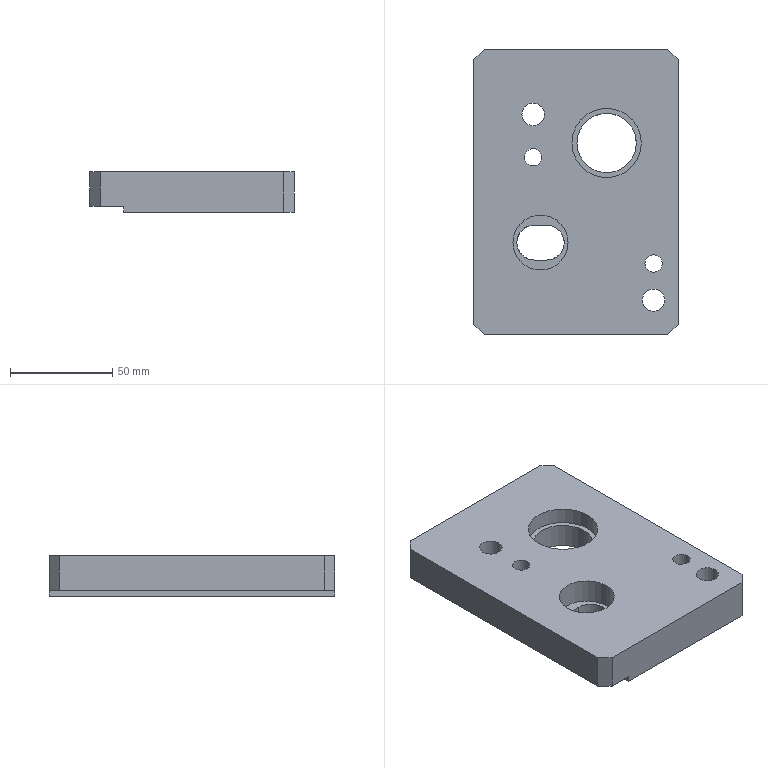Part | STEP file | lll_id3550_x_t | 1 solid | 33 faces | box 100 x 140 x 20 mm | volume 237831 mm3 | plane 20 | cylinder 11 | spline 2 | commonest cylinder face diameters 11 x4 8.5 x2 17 x2 27 x1 29.07 x1 34 x1
STEP:
#1=CARTESIAN_POINT('',(3254.117,145.288,22.5));
#2=VERTEX_POINT('',#1);
#3=CARTESIAN_POINT('',(3258.367,145.288,22.5));
#4=DIRECTION('',(0.,0.,-1.));
#5=DIRECTION('',(-1.,0.,0.));
#6=AXIS2_PLACEMENT_3D('',#3,#4,#5);
#7=CIRCLE('',#6,4.25);
#8=EDGE_CURVE('',#2,#2,#7,.T.);
#9=ORIENTED_EDGE('',*,*,#8,.T.);
#10=EDGE_LOOP('',(#9));
#11=FACE_BOUND('',#10,.T.);
#12=CARTESIAN_POINT('',(3195.117,197.288,22.5));
#13=VERTEX_POINT('',#12);
#14=CARTESIAN_POINT('',(3199.367,197.288,22.5));
#15=DIRECTION('',(0.,0.,-1.));
#16=DIRECTION('',(-1.,0.,0.));
#17=AXIS2_PLACEMENT_3D('',#14,#15,#16);
#18=CIRCLE('',#17,4.25);
#19=EDGE_CURVE('',#13,#13,#18,.T.);
#20=ORIENTED_EDGE('',*,*,#19,.T.);
#21=EDGE_LOOP('',(#20));
#22=FACE_BOUND('',#21,.T.);
#23=CARTESIAN_POINT('',(3252.867,127.288,22.5));
#24=VERTEX_POINT('',#23);
#25=CARTESIAN_POINT('',(3258.367,127.288,22.5));
#26=DIRECTION('',(0.,0.,-1.));
#27=DIRECTION('',(-1.,0.,0.));
#28=AXIS2_PLACEMENT_3D('',#25,#26,#27);
#29=CIRCLE('',#28,5.5);
#30=EDGE_CURVE('',#24,#24,#29,.T.);
#31=ORIENTED_EDGE('',*,*,#30,.T.);
#32=EDGE_LOOP('',(#31));
#33=FACE_BOUND('',#32,.T.);
#34=CARTESIAN_POINT('',(3270.367,115.288,22.5));
#35=VERTEX_POINT('',#34);
#36=CARTESIAN_POINT('',(3270.367,245.288,22.5));
#37=VERTEX_POINT('',#36);
#38=CARTESIAN_POINT('',(3270.367,195.288,22.5));
#39=DIRECTION('',(0.,1.,0.));
#40=VECTOR('',#39,1.);
#41=LINE('',#38,#40);
#42=EDGE_CURVE('',#35,#37,#41,.T.);
#43=ORIENTED_EDGE('',*,*,#42,.T.);
#44=CARTESIAN_POINT('',(3265.367,250.288,22.5));
#45=VERTEX_POINT('',#44);
#46=CARTESIAN_POINT('',(3443.404,72.251,22.5));
#47=DIRECTION('',(-0.7071,0.7071,0.));
#48=VECTOR('',#47,1.);
#49=LINE('',#46,#48);
#50=EDGE_CURVE('',#37,#45,#49,.T.);
#51=ORIENTED_EDGE('',*,*,#50,.T.);
#52=CARTESIAN_POINT('',(3175.367,250.288,22.5));
#53=VERTEX_POINT('',#52);
#54=CARTESIAN_POINT('',(3537.284,250.288,22.5));
#55=DIRECTION('',(-1.,0.,0.));
#56=VECTOR('',#55,1.);
#57=LINE('',#54,#56);
#58=EDGE_CURVE('',#45,#53,#57,.T.);
#59=ORIENTED_EDGE('',*,*,#58,.T.);
#60=CARTESIAN_POINT('',(3170.367,245.288,22.5));
#61=VERTEX_POINT('',#60);
#62=CARTESIAN_POINT('',(3314.247,389.168,22.5));
#63=DIRECTION('',(-0.7071,-0.7071,0.));
#64=VECTOR('',#63,1.);
#65=LINE('',#62,#64);
#66=EDGE_CURVE('',#53,#61,#65,.T.);
#67=ORIENTED_EDGE('',*,*,#66,.T.);
#68=CARTESIAN_POINT('',(3170.367,115.288,22.5));
#69=VERTEX_POINT('',#68);
#70=CARTESIAN_POINT('',(3170.367,166.13,22.5));
#71=DIRECTION('',(0.,1.,0.));
#72=VECTOR('',#71,1.);
#73=LINE('',#70,#72);
#74=EDGE_CURVE('',#69,#61,#73,.T.);
#75=ORIENTED_EDGE('',*,*,#74,.F.);
#76=CARTESIAN_POINT('',(3175.367,110.288,22.5));
#77=VERTEX_POINT('',#76);
#78=CARTESIAN_POINT('',(3328.404,-42.749,22.5));
#79=DIRECTION('',(0.7071,-0.7071,0.));
#80=VECTOR('',#79,1.);
#81=LINE('',#78,#80);
#82=EDGE_CURVE('',#69,#77,#81,.T.);
#83=ORIENTED_EDGE('',*,*,#82,.T.);
#84=CARTESIAN_POINT('',(3265.367,110.288,22.5));
#85=VERTEX_POINT('',#84);
#86=CARTESIAN_POINT('',(3537.284,110.288,22.5));
#87=DIRECTION('',(1.,0.,0.));
#88=VECTOR('',#87,1.);
#89=LINE('',#86,#88);
#90=EDGE_CURVE('',#77,#85,#89,.T.);
#91=ORIENTED_EDGE('',*,*,#90,.T.);
#92=CARTESIAN_POINT('',(3429.247,274.168,22.5));
#93=DIRECTION('',(0.7071,0.7071,0.));
#94=VECTOR('',#93,1.);
#95=LINE('',#92,#94);
#96=EDGE_CURVE('',#85,#35,#95,.T.);
#97=ORIENTED_EDGE('',*,*,#96,.T.);
#98=EDGE_LOOP('',(#43,#51,#59,#67,#75,#83,#91,#97));
#99=FACE_BOUND('',#98,.T.);
#100=CARTESIAN_POINT('',(3193.867,218.288,22.5));
#101=VERTEX_POINT('',#100);
#102=CARTESIAN_POINT('',(3199.367,218.288,22.5));
#103=DIRECTION('',(0.,0.,-1.));
#104=DIRECTION('',(-1.,0.,0.));
#105=AXIS2_PLACEMENT_3D('',#102,#103,#104);
#106=CIRCLE('',#105,5.5);
#107=EDGE_CURVE('',#101,#101,#106,.T.);
#108=ORIENTED_EDGE('',*,*,#107,.T.);
#109=EDGE_LOOP('',(#108));
#110=FACE_BOUND('',#109,.T.);
#111=CARTESIAN_POINT('',(3218.367,204.288,22.5));
#112=VERTEX_POINT('',#111);
#113=CARTESIAN_POINT('',(3235.367,204.288,22.5));
#114=DIRECTION('',(0.,0.,1.));
#115=DIRECTION('',(-1.,0.,0.));
#116=AXIS2_PLACEMENT_3D('',#113,#114,#115);
#117=CIRCLE('',#116,17.);
#118=EDGE_CURVE('',#112,#112,#117,.T.);
#119=ORIENTED_EDGE('',*,*,#118,.F.);
#120=EDGE_LOOP('',(#119));
#121=FACE_BOUND('',#120,.T.);
#122=CARTESIAN_POINT('',(3189.5,155.5,22.5));
#123=VERTEX_POINT('',#122);
#124=CARTESIAN_POINT('',(3203.,155.5,22.5));
#125=DIRECTION('',(0.,0.,-1.));
#126=DIRECTION('',(-1.,0.,0.));
#127=AXIS2_PLACEMENT_3D('',#124,#125,#126);
#128=CIRCLE('',#127,13.5);
#129=EDGE_CURVE('',#123,#123,#128,.T.);
#130=ORIENTED_EDGE('',*,*,#129,.T.);
#131=EDGE_LOOP('',(#130));
#132=FACE_BOUND('',#131,.T.);
#133=CARTESIAN_POINT('',(3537.284,166.13,22.5));
#134=DIRECTION('',(0.,0.,1.));
#135=DIRECTION('',(0.,-1.,0.));
#136=AXIS2_PLACEMENT_3D('',#133,#134,#135);
#137=PLANE('',#136);
#138=ADVANCED_FACE('',(#11,#22,#33,#99,#110,#121,#132),#137,.T.);
#139=CARTESIAN_POINT('',(3220.832,204.288,2.5));
#140=VERTEX_POINT('',#139);
#141=CARTESIAN_POINT('',(3235.367,204.288,2.5));
#142=DIRECTION('',(0.,0.,1.));
#143=DIRECTION('',(-1.,0.,0.));
#144=AXIS2_PLACEMENT_3D('',#141,#142,#143);
#145=CIRCLE('',#144,14.535);
#146=EDGE_CURVE('',#140,#140,#145,.T.);
#147=ORIENTED_EDGE('',*,*,#146,.F.);
#148=EDGE_LOOP('',(#147));
#149=FACE_BOUND('',#148,.T.);
#150=CARTESIAN_POINT('',(3220.832,204.288,14.5));
#151=VERTEX_POINT('',#150);
#152=CARTESIAN_POINT('',(3235.367,204.288,14.5));
#153=DIRECTION('',(0.,0.,1.));
#154=DIRECTION('',(-1.,0.,0.));
#155=AXIS2_PLACEMENT_3D('',#152,#153,#154);
#156=CIRCLE('',#155,14.535);
#157=EDGE_CURVE('',#151,#151,#156,.T.);
#158=ORIENTED_EDGE('',*,*,#157,.T.);
#159=EDGE_LOOP('',(#158));
#160=FACE_BOUND('',#159,.T.);
#161=CARTESIAN_POINT('',(3235.367,204.288,2.5));
#162=DIRECTION('',(0.000000008,0.,-1.));
#163=DIRECTION('',(1.,0.,0.000000008));
#164=AXIS2_PLACEMENT_3D('',#161,#162,#163);
#165=CYLINDRICAL_SURFACE('',#164,14.535);
#166=ADVANCED_FACE('',(#149,#160),#165,.F.);
#167=CARTESIAN_POINT('',(3206.065,146.965,10.5));
#168=VERTEX_POINT('',#167);
#169=CARTESIAN_POINT('',(3199.935,146.965,10.5));
#170=VERTEX_POINT('',#169);
#171=CARTESIAN_POINT('',(3214.,146.965,10.5));
#172=DIRECTION('',(-1.,0.,0.));
#173=VECTOR('',#172,1.);
#174=LINE('',#171,#173);
#175=EDGE_CURVE('',#168,#170,#174,.T.);
#176=ORIENTED_EDGE('',*,*,#175,.F.);
#177=CARTESIAN_POINT('',(3206.065,146.965,2.5));
#178=VERTEX_POINT('',#177);
#179=CARTESIAN_POINT('',(3206.065,146.965,2.5));
#180=DIRECTION('',(-0.000000008,0.,1.));
#181=VECTOR('',#180,1.);
#182=LINE('',#179,#181);
#183=EDGE_CURVE('',#178,#168,#182,.T.);
#184=ORIENTED_EDGE('',*,*,#183,.F.);
#185=CARTESIAN_POINT('',(3199.935,146.965,2.5));
#186=VERTEX_POINT('',#185);
#187=CARTESIAN_POINT('',(3214.,146.965,2.5));
#188=DIRECTION('',(1.,0.,0.));
#189=VECTOR('',#188,1.);
#190=LINE('',#187,#189);
#191=EDGE_CURVE('',#186,#178,#190,.T.);
#192=ORIENTED_EDGE('',*,*,#191,.F.);
#193=CARTESIAN_POINT('',(3199.935,146.965,2.5));
#194=DIRECTION('',(-0.000000008,0.,1.));
#195=VECTOR('',#194,1.);
#196=LINE('',#193,#195);
#197=EDGE_CURVE('',#186,#170,#196,.T.);
#198=ORIENTED_EDGE('',*,*,#197,.T.);
#199=EDGE_LOOP('',(#176,#184,#192,#198));
#200=FACE_OUTER_BOUND('',#199,.T.);
#201=CARTESIAN_POINT('',(3214.,146.965,2.5));
#202=DIRECTION('',(0.,1.,0.));
#203=DIRECTION('',(-1.,0.,-0.000000008));
#204=AXIS2_PLACEMENT_3D('',#201,#202,#203);
#205=PLANE('',#204);
#206=ADVANCED_FACE('',(#200),#205,.T.);
#207=CARTESIAN_POINT('',(3206.065,164.035,10.5));
#208=VERTEX_POINT('',#207);
#209=CARTESIAN_POINT('',(3206.065,164.035,10.5));
#210=CARTESIAN_POINT('',(3208.297,164.035,10.5));
#211=CARTESIAN_POINT('',(3210.515,163.121,10.5));
#212=CARTESIAN_POINT('',(3213.686,159.95,10.5));
#213=CARTESIAN_POINT('',(3214.6,157.741,10.5));
#214=CARTESIAN_POINT('',(3214.6,153.259,10.5));
#215=CARTESIAN_POINT('',(3213.685,151.05,10.5));
#216=CARTESIAN_POINT('',(3210.516,147.88,10.5));
#217=CARTESIAN_POINT('',(3208.297,146.965,10.5));
#218=CARTESIAN_POINT('',(3206.065,146.965,10.5));
#219=B_SPLINE_CURVE_WITH_KNOTS('',3,(#209,#210,#211,#212,#213,#214,#215,#216,#217,#218),.UNSPECIFIED.,.F.,.F.,(4,2,2,2,4),(0.,0.25,0.5,0.75,1.),.UNSPECIFIED.);
#220=EDGE_CURVE('',#208,#168,#219,.T.);
#221=ORIENTED_EDGE('',*,*,#220,.F.);
#222=CARTESIAN_POINT('',(3206.065,164.035,2.5));
#223=VERTEX_POINT('',#222);
#224=CARTESIAN_POINT('',(3206.065,164.035,2.5));
#225=DIRECTION('',(-0.000000008,0.,1.));
#226=VECTOR('',#225,1.);
#227=LINE('',#224,#226);
#228=EDGE_CURVE('',#223,#208,#227,.T.);
#229=ORIENTED_EDGE('',*,*,#228,.F.);
#230=CARTESIAN_POINT('',(3206.065,146.965,2.5));
#231=CARTESIAN_POINT('',(3208.297,146.965,2.5));
#232=CARTESIAN_POINT('',(3210.516,147.88,2.5));
#233=CARTESIAN_POINT('',(3213.685,151.05,2.5));
#234=CARTESIAN_POINT('',(3214.6,153.259,2.5));
#235=CARTESIAN_POINT('',(3214.6,157.741,2.5));
#236=CARTESIAN_POINT('',(3213.686,159.95,2.5));
#237=CARTESIAN_POINT('',(3210.515,163.121,2.5));
#238=CARTESIAN_POINT('',(3208.297,164.035,2.5));
#239=CARTESIAN_POINT('',(3206.065,164.035,2.5));
#240=B_SPLINE_CURVE_WITH_KNOTS('',3,(#230,#231,#232,#233,#234,#235,#236,#237,#238,#239),.UNSPECIFIED.,.F.,.F.,(4,2,2,2,4),(0.,0.25,0.5,0.75,1.),.UNSPECIFIED.);
#241=EDGE_CURVE('',#178,#223,#240,.T.);
#242=ORIENTED_EDGE('',*,*,#241,.F.);
#243=ORIENTED_EDGE('',*,*,#183,.T.);
#244=EDGE_LOOP('',(#221,#229,#242,#243));
#245=FACE_OUTER_BOUND('',#244,.T.);
#246=CARTESIAN_POINT('',(3206.065,164.035,1.5));
#247=CARTESIAN_POINT('',(3206.065,164.035,10.5));
#248=CARTESIAN_POINT('',(3208.297,164.035,1.5));
#249=CARTESIAN_POINT('',(3208.297,164.035,10.5));
#250=CARTESIAN_POINT('',(3210.515,163.121,1.5));
#251=CARTESIAN_POINT('',(3210.515,163.121,10.5));
#252=CARTESIAN_POINT('',(3213.686,159.95,1.5));
#253=CARTESIAN_POINT('',(3213.686,159.95,10.5));
#254=CARTESIAN_POINT('',(3214.6,157.741,1.5));
#255=CARTESIAN_POINT('',(3214.6,157.741,10.5));
#256=CARTESIAN_POINT('',(3214.6,153.259,1.5));
#257=CARTESIAN_POINT('',(3214.6,153.259,10.5));
#258=CARTESIAN_POINT('',(3213.685,151.05,1.5));
#259=CARTESIAN_POINT('',(3213.685,151.05,10.5));
#260=CARTESIAN_POINT('',(3210.516,147.88,1.5));
#261=CARTESIAN_POINT('',(3210.516,147.88,10.5));
#262=CARTESIAN_POINT('',(3208.297,146.965,1.5));
#263=CARTESIAN_POINT('',(3208.297,146.965,10.5));
#264=CARTESIAN_POINT('',(3206.065,146.965,1.5));
#265=CARTESIAN_POINT('',(3206.065,146.965,10.5));
#266=B_SPLINE_SURFACE_WITH_KNOTS('',3,1,((#246,#247),(#248,#249),(#250,#251),(#252,#253),(#254,#255),(#256,#257),(#258,#259),(#260,#261),(#262,#263),(#264,#265)),.UNSPECIFIED.,.F.,.F.,.F.,(4,2,2,2,4),(2,2),(0.,0.25,0.5,0.75,1.),(0.,1.),.UNSPECIFIED.);
#267=ADVANCED_FACE('',(#245),#266,.T.);
#268=CARTESIAN_POINT('',(3199.935,164.035,10.5));
#269=VERTEX_POINT('',#268);
#270=CARTESIAN_POINT('',(3214.,164.035,10.5));
#271=DIRECTION('',(1.,0.,0.));
#272=VECTOR('',#271,1.);
#273=LINE('',#270,#272);
#274=EDGE_CURVE('',#269,#208,#273,.T.);
#275=ORIENTED_EDGE('',*,*,#274,.F.);
#276=CARTESIAN_POINT('',(3199.935,164.035,2.5));
#277=VERTEX_POINT('',#276);
#278=CARTESIAN_POINT('',(3199.935,164.035,2.5));
#279=DIRECTION('',(-0.000000008,0.,1.));
#280=VECTOR('',#279,1.);
#281=LINE('',#278,#280);
#282=EDGE_CURVE('',#277,#269,#281,.T.);
#283=ORIENTED_EDGE('',*,*,#282,.F.);
#284=CARTESIAN_POINT('',(3214.,164.035,2.5));
#285=DIRECTION('',(-1.,0.,0.));
#286=VECTOR('',#285,1.);
#287=LINE('',#284,#286);
#288=EDGE_CURVE('',#223,#277,#287,.T.);
#289=ORIENTED_EDGE('',*,*,#288,.F.);
#290=ORIENTED_EDGE('',*,*,#228,.T.);
#291=EDGE_LOOP('',(#275,#283,#289,#290));
#292=FACE_OUTER_BOUND('',#291,.T.);
#293=CARTESIAN_POINT('',(3214.,164.035,2.5));
#294=DIRECTION('',(0.,-1.,0.));
#295=DIRECTION('',(1.,0.,0.000000008));
#296=AXIS2_PLACEMENT_3D('',#293,#294,#295);
#297=PLANE('',#296);
#298=ADVANCED_FACE('',(#292),#297,.T.);
#299=CARTESIAN_POINT('',(3199.935,146.965,10.5));
#300=CARTESIAN_POINT('',(3197.703,146.965,10.5));
#301=CARTESIAN_POINT('',(3195.485,147.879,10.5));
#302=CARTESIAN_POINT('',(3192.314,151.05,10.5));
#303=CARTESIAN_POINT('',(3191.4,153.259,10.5));
#304=CARTESIAN_POINT('',(3191.4,157.741,10.5));
#305=CARTESIAN_POINT('',(3192.315,159.951,10.5));
#306=CARTESIAN_POINT('',(3195.485,163.12,10.5));
#307=CARTESIAN_POINT('',(3197.703,164.035,10.5));
#308=CARTESIAN_POINT('',(3199.935,164.035,10.5));
#309=B_SPLINE_CURVE_WITH_KNOTS('',3,(#299,#300,#301,#302,#303,#304,#305,#306,#307,#308),.UNSPECIFIED.,.F.,.F.,(4,2,2,2,4),(0.,0.25,0.5,0.75,1.),.UNSPECIFIED.);
#310=EDGE_CURVE('',#170,#269,#309,.T.);
#311=ORIENTED_EDGE('',*,*,#310,.F.);
#312=ORIENTED_EDGE('',*,*,#197,.F.);
#313=CARTESIAN_POINT('',(3199.935,164.035,2.5));
#314=CARTESIAN_POINT('',(3197.703,164.035,2.5));
#315=CARTESIAN_POINT('',(3195.485,163.12,2.5));
#316=CARTESIAN_POINT('',(3192.315,159.951,2.5));
#317=CARTESIAN_POINT('',(3191.4,157.741,2.5));
#318=CARTESIAN_POINT('',(3191.4,153.259,2.5));
#319=CARTESIAN_POINT('',(3192.314,151.05,2.5));
#320=CARTESIAN_POINT('',(3195.485,147.879,2.5));
#321=CARTESIAN_POINT('',(3197.703,146.965,2.5));
#322=CARTESIAN_POINT('',(3199.935,146.965,2.5));
#323=B_SPLINE_CURVE_WITH_KNOTS('',3,(#313,#314,#315,#316,#317,#318,#319,#320,#321,#322),.UNSPECIFIED.,.F.,.F.,(4,2,2,2,4),(0.,0.25,0.5,0.75,1.),.UNSPECIFIED.);
#324=EDGE_CURVE('',#277,#186,#323,.T.);
#325=ORIENTED_EDGE('',*,*,#324,.F.);
#326=ORIENTED_EDGE('',*,*,#282,.T.);
#327=EDGE_LOOP('',(#311,#312,#325,#326));
#328=FACE_OUTER_BOUND('',#327,.T.);
#329=CARTESIAN_POINT('',(3199.935,146.965,1.5));
#330=CARTESIAN_POINT('',(3199.935,146.965,10.5));
#331=CARTESIAN_POINT('',(3197.703,146.965,1.5));
#332=CARTESIAN_POINT('',(3197.703,146.965,10.5));
#333=CARTESIAN_POINT('',(3195.485,147.879,1.5));
#334=CARTESIAN_POINT('',(3195.485,147.879,10.5));
#335=CARTESIAN_POINT('',(3192.314,151.05,1.5));
#336=CARTESIAN_POINT('',(3192.314,151.05,10.5));
#337=CARTESIAN_POINT('',(3191.4,153.259,1.5));
#338=CARTESIAN_POINT('',(3191.4,153.259,10.5));
#339=CARTESIAN_POINT('',(3191.4,157.741,1.5));
#340=CARTESIAN_POINT('',(3191.4,157.741,10.5));
#341=CARTESIAN_POINT('',(3192.315,159.951,1.5));
#342=CARTESIAN_POINT('',(3192.315,159.951,10.5));
#343=CARTESIAN_POINT('',(3195.485,163.12,1.5));
#344=CARTESIAN_POINT('',(3195.485,163.12,10.5));
#345=CARTESIAN_POINT('',(3197.703,164.035,1.5));
#346=CARTESIAN_POINT('',(3197.703,164.035,10.5));
#347=CARTESIAN_POINT('',(3199.935,164.035,1.5));
#348=CARTESIAN_POINT('',(3199.935,164.035,10.5));
#349=B_SPLINE_SURFACE_WITH_KNOTS('',3,1,((#329,#330),(#331,#332),(#333,#334),(#335,#336),(#337,#338),(#339,#340),(#341,#342),(#343,#344),(#345,#346),(#347,#348)),.UNSPECIFIED.,.F.,.F.,.F.,(4,2,2,2,4),(2,2),(0.,0.25,0.5,0.75,1.),(0.,1.),.UNSPECIFIED.);
#350=ADVANCED_FACE('',(#328),#349,.T.);
#351=CARTESIAN_POINT('',(3186.89,250.288,2.5));
#352=VERTEX_POINT('',#351);
#353=CARTESIAN_POINT('',(3265.367,250.288,2.5));
#354=VERTEX_POINT('',#353);
#355=CARTESIAN_POINT('',(3227.867,250.288,2.5));
#356=DIRECTION('',(1.,0.,0.));
#357=VECTOR('',#356,1.);
#358=LINE('',#355,#357);
#359=EDGE_CURVE('',#352,#354,#358,.T.);
#360=ORIENTED_EDGE('',*,*,#359,.T.);
#361=CARTESIAN_POINT('',(3270.367,245.288,2.5));
#362=VERTEX_POINT('',#361);
#363=CARTESIAN_POINT('',(3270.367,245.288,2.5));
#364=DIRECTION('',(0.7071,-0.7071,0.));
#365=VECTOR('',#364,1.);
#366=LINE('',#363,#365);
#367=EDGE_CURVE('',#354,#362,#366,.T.);
#368=ORIENTED_EDGE('',*,*,#367,.T.);
#369=CARTESIAN_POINT('',(3270.367,115.288,2.5));
#370=VERTEX_POINT('',#369);
#371=CARTESIAN_POINT('',(3270.367,195.288,2.5));
#372=DIRECTION('',(0.,-1.,0.));
#373=VECTOR('',#372,1.);
#374=LINE('',#371,#373);
#375=EDGE_CURVE('',#362,#370,#374,.T.);
#376=ORIENTED_EDGE('',*,*,#375,.T.);
#377=CARTESIAN_POINT('',(3265.367,110.288,2.5));
#378=VERTEX_POINT('',#377);
#379=CARTESIAN_POINT('',(3265.367,110.288,2.5));
#380=DIRECTION('',(-0.7071,-0.7071,0.));
#381=VECTOR('',#380,1.);
#382=LINE('',#379,#381);
#383=EDGE_CURVE('',#370,#378,#382,.T.);
#384=ORIENTED_EDGE('',*,*,#383,.T.);
#385=CARTESIAN_POINT('',(3186.89,110.288,2.5));
#386=VERTEX_POINT('',#385);
#387=CARTESIAN_POINT('',(3227.867,110.288,2.5));
#388=DIRECTION('',(-1.,0.,0.));
#389=VECTOR('',#388,1.);
#390=LINE('',#387,#389);
#391=EDGE_CURVE('',#378,#386,#390,.T.);
#392=ORIENTED_EDGE('',*,*,#391,.T.);
#393=CARTESIAN_POINT('',(3186.89,0.,2.5));
#394=DIRECTION('',(0.,1.,0.));
#395=VECTOR('',#394,1.);
#396=LINE('',#393,#395);
#397=EDGE_CURVE('',#386,#352,#396,.T.);
#398=ORIENTED_EDGE('',*,*,#397,.T.);
#399=EDGE_LOOP('',(#360,#368,#376,#384,#392,#398));
#400=FACE_BOUND('',#399,.T.);
#401=CARTESIAN_POINT('',(3193.867,197.288,2.5));
#402=VERTEX_POINT('',#401);
#403=CARTESIAN_POINT('',(3199.367,197.288,2.5));
#404=DIRECTION('',(0.,0.,-1.));
#405=DIRECTION('',(-1.,0.,0.));
#406=AXIS2_PLACEMENT_3D('',#403,#404,#405);
#407=CIRCLE('',#406,5.5);
#408=EDGE_CURVE('',#402,#402,#407,.T.);
#409=ORIENTED_EDGE('',*,*,#408,.F.);
#410=EDGE_LOOP('',(#409));
#411=FACE_BOUND('',#410,.T.);
#412=ORIENTED_EDGE('',*,*,#146,.T.);
#413=EDGE_LOOP('',(#412));
#414=FACE_BOUND('',#413,.T.);
#415=CARTESIAN_POINT('',(3249.867,127.288,2.5));
#416=VERTEX_POINT('',#415);
#417=CARTESIAN_POINT('',(3258.367,127.288,2.5));
#418=DIRECTION('',(0.,0.,1.));
#419=DIRECTION('',(-1.,0.,0.));
#420=AXIS2_PLACEMENT_3D('',#417,#418,#419);
#421=CIRCLE('',#420,8.5);
#422=EDGE_CURVE('',#416,#416,#421,.T.);
#423=ORIENTED_EDGE('',*,*,#422,.T.);
#424=EDGE_LOOP('',(#423));
#425=FACE_BOUND('',#424,.T.);
#426=CARTESIAN_POINT('',(3252.867,145.288,2.5));
#427=VERTEX_POINT('',#426);
#428=CARTESIAN_POINT('',(3258.367,145.288,2.5));
#429=DIRECTION('',(0.,0.,1.));
#430=DIRECTION('',(-1.,0.,0.));
#431=AXIS2_PLACEMENT_3D('',#428,#429,#430);
#432=CIRCLE('',#431,5.5);
#433=EDGE_CURVE('',#427,#427,#432,.T.);
#434=ORIENTED_EDGE('',*,*,#433,.T.);
#435=EDGE_LOOP('',(#434));
#436=FACE_BOUND('',#435,.T.);
#437=CARTESIAN_POINT('',(3190.867,218.288,2.5));
#438=VERTEX_POINT('',#437);
#439=CARTESIAN_POINT('',(3199.367,218.288,2.5));
#440=DIRECTION('',(0.,0.,-1.));
#441=DIRECTION('',(-1.,0.,0.));
#442=AXIS2_PLACEMENT_3D('',#439,#440,#441);
#443=CIRCLE('',#442,8.5);
#444=EDGE_CURVE('',#438,#438,#443,.T.);
#445=ORIENTED_EDGE('',*,*,#444,.F.);
#446=EDGE_LOOP('',(#445));
#447=FACE_BOUND('',#446,.T.);
#448=ORIENTED_EDGE('',*,*,#324,.T.);
#449=ORIENTED_EDGE('',*,*,#191,.T.);
#450=ORIENTED_EDGE('',*,*,#241,.T.);
#451=ORIENTED_EDGE('',*,*,#288,.T.);
#452=EDGE_LOOP('',(#448,#449,#450,#451));
#453=FACE_BOUND('',#452,.T.);
#454=CARTESIAN_POINT('',(2132.435,0.,2.5));
#455=DIRECTION('',(0.,0.,-1.));
#456=DIRECTION('',(-1.,0.,0.));
#457=AXIS2_PLACEMENT_3D('',#454,#455,#456);
#458=PLANE('',#457);
#459=ADVANCED_FACE('',(#400,#411,#414,#425,#436,#447,#453),#458,.T.);
#460=CARTESIAN_POINT('',(3193.867,197.288,9.5));
#461=VERTEX_POINT('',#460);
#462=CARTESIAN_POINT('',(3199.367,197.288,9.5));
#463=DIRECTION('',(0.,0.,1.));
#464=DIRECTION('',(-1.,0.,0.));
#465=AXIS2_PLACEMENT_3D('',#462,#463,#464);
#466=CIRCLE('',#465,5.5);
#467=EDGE_CURVE('',#461,#461,#466,.T.);
#468=ORIENTED_EDGE('',*,*,#467,.T.);
#469=EDGE_LOOP('',(#468));
#470=FACE_BOUND('',#469,.T.);
#471=ORIENTED_EDGE('',*,*,#408,.T.);
#472=EDGE_LOOP('',(#471));
#473=FACE_BOUND('',#472,.T.);
#474=CARTESIAN_POINT('',(3199.367,197.288,-2.5));
#475=DIRECTION('',(0.,0.,1.));
#476=DIRECTION('',(-1.,0.,0.));
#477=AXIS2_PLACEMENT_3D('',#474,#475,#476);
#478=CYLINDRICAL_SURFACE('',#477,5.5);
#479=ADVANCED_FACE('',(#470,#473),#478,.F.);
#480=ORIENTED_EDGE('',*,*,#391,.F.);
#481=CARTESIAN_POINT('',(3265.367,110.288,-81.5));
#482=DIRECTION('',(0.,0.,1.));
#483=VECTOR('',#482,1.);
#484=LINE('',#481,#483);
#485=EDGE_CURVE('',#378,#85,#484,.T.);
#486=ORIENTED_EDGE('',*,*,#485,.T.);
#487=ORIENTED_EDGE('',*,*,#90,.F.);
#488=CARTESIAN_POINT('',(3175.367,110.288,5.398));
#489=VERTEX_POINT('',#488);
#490=CARTESIAN_POINT('',(3175.367,110.288,-81.5));
#491=DIRECTION('',(0.,0.,-1.));
#492=VECTOR('',#491,1.);
#493=LINE('',#490,#492);
#494=EDGE_CURVE('',#77,#489,#493,.T.);
#495=ORIENTED_EDGE('',*,*,#494,.T.);
#496=CARTESIAN_POINT('',(3186.89,110.288,5.398));
#497=VERTEX_POINT('',#496);
#498=CARTESIAN_POINT('',(3227.867,110.288,5.398));
#499=DIRECTION('',(-1.,0.,0.));
#500=VECTOR('',#499,1.);
#501=LINE('',#498,#500);
#502=EDGE_CURVE('',#497,#489,#501,.T.);
#503=ORIENTED_EDGE('',*,*,#502,.F.);
#504=CARTESIAN_POINT('',(3186.89,110.288,-81.5));
#505=DIRECTION('',(0.,0.,1.));
#506=VECTOR('',#505,1.);
#507=LINE('',#504,#506);
#508=EDGE_CURVE('',#386,#497,#507,.T.);
#509=ORIENTED_EDGE('',*,*,#508,.F.);
#510=EDGE_LOOP('',(#480,#486,#487,#495,#503,#509));
#511=FACE_OUTER_BOUND('',#510,.T.);
#512=CARTESIAN_POINT('',(3227.867,110.288,-81.5));
#513=DIRECTION('',(0.,-1.,0.));
#514=DIRECTION('',(0.,0.,-1.));
#515=AXIS2_PLACEMENT_3D('',#512,#513,#514);
#516=PLANE('',#515);
#517=ADVANCED_FACE('',(#511),#516,.T.);
#518=ORIENTED_EDGE('',*,*,#74,.T.);
#519=CARTESIAN_POINT('',(3170.367,245.288,5.398));
#520=VERTEX_POINT('',#519);
#521=CARTESIAN_POINT('',(3170.367,245.288,13.5));
#522=DIRECTION('',(0.,0.,-1.));
#523=VECTOR('',#522,1.);
#524=LINE('',#521,#523);
#525=EDGE_CURVE('',#61,#520,#524,.T.);
#526=ORIENTED_EDGE('',*,*,#525,.T.);
#527=CARTESIAN_POINT('',(3170.367,115.288,5.398));
#528=VERTEX_POINT('',#527);
#529=CARTESIAN_POINT('',(3170.367,195.288,5.398));
#530=DIRECTION('',(0.,-1.,0.));
#531=VECTOR('',#530,1.);
#532=LINE('',#529,#531);
#533=EDGE_CURVE('',#520,#528,#532,.T.);
#534=ORIENTED_EDGE('',*,*,#533,.T.);
#535=CARTESIAN_POINT('',(3170.367,115.288,13.5));
#536=DIRECTION('',(0.,0.,1.));
#537=VECTOR('',#536,1.);
#538=LINE('',#535,#537);
#539=EDGE_CURVE('',#528,#69,#538,.T.);
#540=ORIENTED_EDGE('',*,*,#539,.T.);
#541=EDGE_LOOP('',(#518,#526,#534,#540));
#542=FACE_OUTER_BOUND('',#541,.T.);
#543=CARTESIAN_POINT('',(3170.367,195.288,13.5));
#544=DIRECTION('',(-1.,0.,0.));
#545=DIRECTION('',(0.,0.,1.));
#546=AXIS2_PLACEMENT_3D('',#543,#544,#545);
#547=PLANE('',#546);
#548=ADVANCED_FACE('',(#542),#547,.T.);
#549=ORIENTED_EDGE('',*,*,#58,.F.);
#550=CARTESIAN_POINT('',(3265.367,250.288,-81.5));
#551=DIRECTION('',(0.,0.,-1.));
#552=VECTOR('',#551,1.);
#553=LINE('',#550,#552);
#554=EDGE_CURVE('',#45,#354,#553,.T.);
#555=ORIENTED_EDGE('',*,*,#554,.T.);
#556=ORIENTED_EDGE('',*,*,#359,.F.);
#557=CARTESIAN_POINT('',(3186.89,250.288,5.398));
#558=VERTEX_POINT('',#557);
#559=CARTESIAN_POINT('',(3186.89,250.288,2.5));
#560=DIRECTION('',(0.,0.,1.));
#561=VECTOR('',#560,1.);
#562=LINE('',#559,#561);
#563=EDGE_CURVE('',#352,#558,#562,.T.);
#564=ORIENTED_EDGE('',*,*,#563,.T.);
#565=CARTESIAN_POINT('',(3175.367,250.288,5.398));
#566=VERTEX_POINT('',#565);
#567=CARTESIAN_POINT('',(3227.867,250.288,5.398));
#568=DIRECTION('',(1.,0.,0.));
#569=VECTOR('',#568,1.);
#570=LINE('',#567,#569);
#571=EDGE_CURVE('',#566,#558,#570,.T.);
#572=ORIENTED_EDGE('',*,*,#571,.F.);
#573=CARTESIAN_POINT('',(3175.367,250.288,-81.5));
#574=DIRECTION('',(0.,0.,1.));
#575=VECTOR('',#574,1.);
#576=LINE('',#573,#575);
#577=EDGE_CURVE('',#566,#53,#576,.T.);
#578=ORIENTED_EDGE('',*,*,#577,.T.);
#579=EDGE_LOOP('',(#549,#555,#556,#564,#572,#578));
#580=FACE_OUTER_BOUND('',#579,.T.);
#581=CARTESIAN_POINT('',(3227.867,250.288,-81.5));
#582=DIRECTION('',(0.,1.,0.));
#583=DIRECTION('',(0.,0.,1.));
#584=AXIS2_PLACEMENT_3D('',#581,#582,#583);
#585=PLANE('',#584);
#586=ADVANCED_FACE('',(#580),#585,.T.);
#587=CARTESIAN_POINT('',(3190.867,218.288,14.5));
#588=VERTEX_POINT('',#587);
#589=CARTESIAN_POINT('',(3199.367,218.288,14.5));
#590=DIRECTION('',(0.,0.,1.));
#591=DIRECTION('',(-1.,0.,0.));
#592=AXIS2_PLACEMENT_3D('',#589,#590,#591);
#593=CIRCLE('',#592,8.5);
#594=EDGE_CURVE('',#588,#588,#593,.T.);
#595=ORIENTED_EDGE('',*,*,#594,.T.);
#596=EDGE_LOOP('',(#595));
#597=FACE_BOUND('',#596,.T.);
#598=ORIENTED_EDGE('',*,*,#444,.T.);
#599=EDGE_LOOP('',(#598));
#600=FACE_BOUND('',#599,.T.);
#601=CARTESIAN_POINT('',(3199.367,218.288,-2.5));
#602=DIRECTION('',(0.,0.,1.));
#603=DIRECTION('',(0.,-1.,0.));
#604=AXIS2_PLACEMENT_3D('',#601,#602,#603);
#605=CYLINDRICAL_SURFACE('',#604,8.5);
#606=ADVANCED_FACE('',(#597,#600),#605,.F.);
#607=CARTESIAN_POINT('',(3195.117,197.288,9.5));
#608=VERTEX_POINT('',#607);
#609=CARTESIAN_POINT('',(3199.367,197.288,9.5));
#610=DIRECTION('',(0.,0.,1.));
#611=DIRECTION('',(-1.,0.,0.));
#612=AXIS2_PLACEMENT_3D('',#609,#610,#611);
#613=CIRCLE('',#612,4.25);
#614=EDGE_CURVE('',#608,#608,#613,.T.);
#615=ORIENTED_EDGE('',*,*,#614,.T.);
#616=EDGE_LOOP('',(#615));
#617=FACE_BOUND('',#616,.T.);
#618=ORIENTED_EDGE('',*,*,#467,.F.);
#619=EDGE_LOOP('',(#618));
#620=FACE_BOUND('',#619,.T.);
#621=CARTESIAN_POINT('',(3195.367,197.288,9.5));
#622=DIRECTION('',(0.,0.,1.));
#623=DIRECTION('',(-1.,0.,0.));
#624=AXIS2_PLACEMENT_3D('',#621,#622,#623);
#625=PLANE('',#624);
#626=ADVANCED_FACE('',(#617,#620),#625,.F.);
#627=CARTESIAN_POINT('',(3252.867,127.288,14.5));
#628=VERTEX_POINT('',#627);
#629=CARTESIAN_POINT('',(3258.367,127.288,14.5));
#630=DIRECTION('',(0.,0.,-1.));
#631=DIRECTION('',(-1.,0.,0.));
#632=AXIS2_PLACEMENT_3D('',#629,#630,#631);
#633=CIRCLE('',#632,5.5);
#634=EDGE_CURVE('',#628,#628,#633,.T.);
#635=ORIENTED_EDGE('',*,*,#634,.F.);
#636=EDGE_LOOP('',(#635));
#637=FACE_BOUND('',#636,.T.);
#638=CARTESIAN_POINT('',(3249.867,127.288,14.5));
#639=VERTEX_POINT('',#638);
#640=CARTESIAN_POINT('',(3258.367,127.288,14.5));
#641=DIRECTION('',(0.,0.,-1.));
#642=DIRECTION('',(-1.,0.,0.));
#643=AXIS2_PLACEMENT_3D('',#640,#641,#642);
#644=CIRCLE('',#643,8.5);
#645=EDGE_CURVE('',#639,#639,#644,.T.);
#646=ORIENTED_EDGE('',*,*,#645,.T.);
#647=EDGE_LOOP('',(#646));
#648=FACE_BOUND('',#647,.T.);
#649=CARTESIAN_POINT('',(3258.367,127.288,14.5));
#650=DIRECTION('',(0.,0.,1.));
#651=DIRECTION('',(0.,1.,0.));
#652=AXIS2_PLACEMENT_3D('',#649,#650,#651);
#653=PLANE('',#652);
#654=ADVANCED_FACE('',(#637,#648),#653,.F.);
#655=CARTESIAN_POINT('',(3193.867,218.288,14.5));
#656=VERTEX_POINT('',#655);
#657=CARTESIAN_POINT('',(3199.367,218.288,14.5));
#658=DIRECTION('',(0.,0.,1.));
#659=DIRECTION('',(-1.,0.,0.));
#660=AXIS2_PLACEMENT_3D('',#657,#658,#659);
#661=CIRCLE('',#660,5.5);
#662=EDGE_CURVE('',#656,#656,#661,.T.);
#663=ORIENTED_EDGE('',*,*,#662,.T.);
#664=EDGE_LOOP('',(#663));
#665=FACE_BOUND('',#664,.T.);
#666=ORIENTED_EDGE('',*,*,#594,.F.);
#667=EDGE_LOOP('',(#666));
#668=FACE_BOUND('',#667,.T.);
#669=CARTESIAN_POINT('',(3195.367,218.288,14.5));
#670=DIRECTION('',(0.,0.,1.));
#671=DIRECTION('',(0.,-1.,0.));
#672=AXIS2_PLACEMENT_3D('',#669,#670,#671);
#673=PLANE('',#672);
#674=ADVANCED_FACE('',(#665,#668),#673,.F.);
#675=ORIENTED_EDGE('',*,*,#107,.F.);
#676=EDGE_LOOP('',(#675));
#677=FACE_BOUND('',#676,.T.);
#678=ORIENTED_EDGE('',*,*,#662,.F.);
#679=EDGE_LOOP('',(#678));
#680=FACE_BOUND('',#679,.T.);
#681=CARTESIAN_POINT('',(3199.367,218.288,97.5));
#682=DIRECTION('',(0.,0.,1.));
#683=DIRECTION('',(0.,-1.,0.));
#684=AXIS2_PLACEMENT_3D('',#681,#682,#683);
#685=CYLINDRICAL_SURFACE('',#684,5.5);
#686=ADVANCED_FACE('',(#677,#680),#685,.F.);
#687=ORIENTED_EDGE('',*,*,#645,.F.);
#688=EDGE_LOOP('',(#687));
#689=FACE_BOUND('',#688,.T.);
#690=ORIENTED_EDGE('',*,*,#422,.F.);
#691=EDGE_LOOP('',(#690));
#692=FACE_BOUND('',#691,.T.);
#693=CARTESIAN_POINT('',(3258.367,127.288,-2.5));
#694=DIRECTION('',(0.,0.,1.));
#695=DIRECTION('',(0.,1.,0.));
#696=AXIS2_PLACEMENT_3D('',#693,#694,#695);
#697=CYLINDRICAL_SURFACE('',#696,8.5);
#698=ADVANCED_FACE('',(#689,#692),#697,.F.);
#699=ORIENTED_EDGE('',*,*,#375,.F.);
#700=CARTESIAN_POINT('',(3270.367,245.288,-81.5));
#701=DIRECTION('',(0.,0.,1.));
#702=VECTOR('',#701,1.);
#703=LINE('',#700,#702);
#704=EDGE_CURVE('',#362,#37,#703,.T.);
#705=ORIENTED_EDGE('',*,*,#704,.T.);
#706=ORIENTED_EDGE('',*,*,#42,.F.);
#707=CARTESIAN_POINT('',(3270.367,115.288,-81.5));
#708=DIRECTION('',(0.,0.,-1.));
#709=VECTOR('',#708,1.);
#710=LINE('',#707,#709);
#711=EDGE_CURVE('',#35,#370,#710,.T.);
#712=ORIENTED_EDGE('',*,*,#711,.T.);
#713=EDGE_LOOP('',(#699,#705,#706,#712));
#714=FACE_OUTER_BOUND('',#713,.T.);
#715=CARTESIAN_POINT('',(3270.367,195.288,-81.5));
#716=DIRECTION('',(1.,0.,0.));
#717=DIRECTION('',(0.,0.,-1.));
#718=AXIS2_PLACEMENT_3D('',#715,#716,#717);
#719=PLANE('',#718);
#720=ADVANCED_FACE('',(#714),#719,.T.);
#721=ORIENTED_EDGE('',*,*,#30,.F.);
#722=EDGE_LOOP('',(#721));
#723=FACE_BOUND('',#722,.T.);
#724=ORIENTED_EDGE('',*,*,#634,.T.);
#725=EDGE_LOOP('',(#724));
#726=FACE_BOUND('',#725,.T.);
#727=CARTESIAN_POINT('',(3258.367,127.288,97.5));
#728=DIRECTION('',(0.,0.,1.));
#729=DIRECTION('',(0.,1.,0.));
#730=AXIS2_PLACEMENT_3D('',#727,#728,#729);
#731=CYLINDRICAL_SURFACE('',#730,5.5);
#732=ADVANCED_FACE('',(#723,#726),#731,.F.);
#733=ORIENTED_EDGE('',*,*,#19,.F.);
#734=EDGE_LOOP('',(#733));
#735=FACE_BOUND('',#734,.T.);
#736=ORIENTED_EDGE('',*,*,#614,.F.);
#737=EDGE_LOOP('',(#736));
#738=FACE_BOUND('',#737,.T.);
#739=CARTESIAN_POINT('',(3199.367,197.288,97.5));
#740=DIRECTION('',(0.,0.,1.));
#741=DIRECTION('',(-1.,0.,0.));
#742=AXIS2_PLACEMENT_3D('',#739,#740,#741);
#743=CYLINDRICAL_SURFACE('',#742,4.25);
#744=ADVANCED_FACE('',(#735,#738),#743,.F.);
#745=ORIENTED_EDGE('',*,*,#8,.F.);
#746=EDGE_LOOP('',(#745));
#747=FACE_BOUND('',#746,.T.);
#748=CARTESIAN_POINT('',(3254.117,145.288,9.5));
#749=VERTEX_POINT('',#748);
#750=CARTESIAN_POINT('',(3258.367,145.288,9.5));
#751=DIRECTION('',(0.,0.,1.));
#752=DIRECTION('',(-1.,0.,0.));
#753=AXIS2_PLACEMENT_3D('',#750,#751,#752);
#754=CIRCLE('',#753,4.25);
#755=EDGE_CURVE('',#749,#749,#754,.T.);
#756=ORIENTED_EDGE('',*,*,#755,.F.);
#757=EDGE_LOOP('',(#756));
#758=FACE_BOUND('',#757,.T.);
#759=CARTESIAN_POINT('',(3258.367,145.288,97.5));
#760=DIRECTION('',(0.,0.,1.));
#761=DIRECTION('',(1.,0.,0.));
#762=AXIS2_PLACEMENT_3D('',#759,#760,#761);
#763=CYLINDRICAL_SURFACE('',#762,4.25);
#764=ADVANCED_FACE('',(#747,#758),#763,.F.);
#765=ORIENTED_EDGE('',*,*,#755,.T.);
#766=EDGE_LOOP('',(#765));
#767=FACE_BOUND('',#766,.T.);
#768=CARTESIAN_POINT('',(3252.867,145.288,9.5));
#769=VERTEX_POINT('',#768);
#770=CARTESIAN_POINT('',(3258.367,145.288,9.5));
#771=DIRECTION('',(0.,0.,1.));
#772=DIRECTION('',(-1.,0.,0.));
#773=AXIS2_PLACEMENT_3D('',#770,#771,#772);
#774=CIRCLE('',#773,5.5);
#775=EDGE_CURVE('',#769,#769,#774,.T.);
#776=ORIENTED_EDGE('',*,*,#775,.F.);
#777=EDGE_LOOP('',(#776));
#778=FACE_BOUND('',#777,.T.);
#779=CARTESIAN_POINT('',(3258.367,145.288,9.5));
#780=DIRECTION('',(0.,0.,1.));
#781=DIRECTION('',(1.,0.,0.));
#782=AXIS2_PLACEMENT_3D('',#779,#780,#781);
#783=PLANE('',#782);
#784=ADVANCED_FACE('',(#767,#778),#783,.F.);
#785=ORIENTED_EDGE('',*,*,#775,.T.);
#786=EDGE_LOOP('',(#785));
#787=FACE_BOUND('',#786,.T.);
#788=ORIENTED_EDGE('',*,*,#433,.F.);
#789=EDGE_LOOP('',(#788));
#790=FACE_BOUND('',#789,.T.);
#791=CARTESIAN_POINT('',(3258.367,145.288,-2.5));
#792=DIRECTION('',(0.,0.,1.));
#793=DIRECTION('',(1.,0.,0.));
#794=AXIS2_PLACEMENT_3D('',#791,#792,#793);
#795=CYLINDRICAL_SURFACE('',#794,5.5);
#796=ADVANCED_FACE('',(#787,#790),#795,.F.);
#797=ORIENTED_EDGE('',*,*,#118,.T.);
#798=EDGE_LOOP('',(#797));
#799=FACE_BOUND('',#798,.T.);
#800=CARTESIAN_POINT('',(3218.367,204.288,14.5));
#801=VERTEX_POINT('',#800);
#802=CARTESIAN_POINT('',(3235.367,204.288,14.5));
#803=DIRECTION('',(0.,0.,-1.));
#804=DIRECTION('',(-1.,0.,0.));
#805=AXIS2_PLACEMENT_3D('',#802,#803,#804);
#806=CIRCLE('',#805,17.);
#807=EDGE_CURVE('',#801,#801,#806,.T.);
#808=ORIENTED_EDGE('',*,*,#807,.T.);
#809=EDGE_LOOP('',(#808));
#810=FACE_BOUND('',#809,.T.);
#811=CARTESIAN_POINT('',(3235.367,204.288,14.5));
#812=DIRECTION('',(0.,0.,1.));
#813=DIRECTION('',(-1.,0.,0.));
#814=AXIS2_PLACEMENT_3D('',#811,#812,#813);
#815=CYLINDRICAL_SURFACE('',#814,17.);
#816=ADVANCED_FACE('',(#799,#810),#815,.F.);
#817=ORIENTED_EDGE('',*,*,#157,.F.);
#818=EDGE_LOOP('',(#817));
#819=FACE_BOUND('',#818,.T.);
#820=ORIENTED_EDGE('',*,*,#807,.F.);
#821=EDGE_LOOP('',(#820));
#822=FACE_BOUND('',#821,.T.);
#823=CARTESIAN_POINT('',(3235.367,204.288,14.5));
#824=DIRECTION('',(0.,0.,1.));
#825=DIRECTION('',(-1.,0.,0.));
#826=AXIS2_PLACEMENT_3D('',#823,#824,#825);
#827=PLANE('',#826);
#828=ADVANCED_FACE('',(#819,#822),#827,.T.);
#829=ORIENTED_EDGE('',*,*,#129,.F.);
#830=EDGE_LOOP('',(#829));
#831=FACE_BOUND('',#830,.T.);
#832=CARTESIAN_POINT('',(3216.5,155.5,10.5));
#833=VERTEX_POINT('',#832);
#834=CARTESIAN_POINT('',(3203.,155.5,10.5));
#835=DIRECTION('',(0.,0.,1.));
#836=DIRECTION('',(1.,0.,0.));
#837=AXIS2_PLACEMENT_3D('',#834,#835,#836);
#838=CIRCLE('',#837,13.5);
#839=EDGE_CURVE('',#833,#833,#838,.T.);
#840=ORIENTED_EDGE('',*,*,#839,.F.);
#841=EDGE_LOOP('',(#840));
#842=FACE_BOUND('',#841,.T.);
#843=CARTESIAN_POINT('',(3203.,155.5,14.5));
#844=DIRECTION('',(0.,0.,1.));
#845=DIRECTION('',(-1.,0.,0.));
#846=AXIS2_PLACEMENT_3D('',#843,#844,#845);
#847=CYLINDRICAL_SURFACE('',#846,13.5);
#848=ADVANCED_FACE('',(#831,#842),#847,.F.);
#849=ORIENTED_EDGE('',*,*,#175,.T.);
#850=ORIENTED_EDGE('',*,*,#310,.T.);
#851=ORIENTED_EDGE('',*,*,#274,.T.);
#852=ORIENTED_EDGE('',*,*,#220,.T.);
#853=EDGE_LOOP('',(#849,#850,#851,#852));
#854=FACE_BOUND('',#853,.T.);
#855=ORIENTED_EDGE('',*,*,#839,.T.);
#856=EDGE_LOOP('',(#855));
#857=FACE_BOUND('',#856,.T.);
#858=CARTESIAN_POINT('',(3203.,155.5,10.5));
#859=DIRECTION('',(0.,0.,-1.));
#860=DIRECTION('',(1.,0.,0.));
#861=AXIS2_PLACEMENT_3D('',#858,#859,#860);
#862=PLANE('',#861);
#863=ADVANCED_FACE('',(#854,#857),#862,.F.);
#864=CARTESIAN_POINT('',(3186.89,185.288,5.398));
#865=DIRECTION('',(0.,1.,0.));
#866=VECTOR('',#865,1.);
#867=LINE('',#864,#866);
#868=EDGE_CURVE('',#497,#558,#867,.T.);
#869=ORIENTED_EDGE('',*,*,#868,.T.);
#870=ORIENTED_EDGE('',*,*,#563,.F.);
#871=ORIENTED_EDGE('',*,*,#397,.F.);
#872=ORIENTED_EDGE('',*,*,#508,.T.);
#873=EDGE_LOOP('',(#869,#870,#871,#872));
#874=FACE_OUTER_BOUND('',#873,.T.);
#875=CARTESIAN_POINT('',(3186.89,185.288,2.5));
#876=DIRECTION('',(1.,0.,0.));
#877=DIRECTION('',(0.,0.,-1.));
#878=AXIS2_PLACEMENT_3D('',#875,#876,#877);
#879=PLANE('',#878);
#880=ADVANCED_FACE('',(#874),#879,.F.);
#881=ORIENTED_EDGE('',*,*,#533,.F.);
#882=CARTESIAN_POINT('',(3170.367,245.288,5.398));
#883=DIRECTION('',(0.7071,0.7071,0.));
#884=VECTOR('',#883,1.);
#885=LINE('',#882,#884);
#886=EDGE_CURVE('',#520,#566,#885,.T.);
#887=ORIENTED_EDGE('',*,*,#886,.T.);
#888=ORIENTED_EDGE('',*,*,#571,.T.);
#889=ORIENTED_EDGE('',*,*,#868,.F.);
#890=ORIENTED_EDGE('',*,*,#502,.T.);
#891=CARTESIAN_POINT('',(3175.367,110.288,5.398));
#892=DIRECTION('',(-0.7071,0.7071,0.));
#893=VECTOR('',#892,1.);
#894=LINE('',#891,#893);
#895=EDGE_CURVE('',#489,#528,#894,.T.);
#896=ORIENTED_EDGE('',*,*,#895,.T.);
#897=EDGE_LOOP('',(#881,#887,#888,#889,#890,#896));
#898=FACE_OUTER_BOUND('',#897,.T.);
#899=CARTESIAN_POINT('',(3178.628,185.288,5.398));
#900=DIRECTION('',(0.,0.,1.));
#901=DIRECTION('',(1.,0.,0.));
#902=AXIS2_PLACEMENT_3D('',#899,#900,#901);
#903=PLANE('',#902);
#904=ADVANCED_FACE('',(#898),#903,.F.);
#905=ORIENTED_EDGE('',*,*,#383,.F.);
#906=ORIENTED_EDGE('',*,*,#711,.F.);
#907=ORIENTED_EDGE('',*,*,#96,.F.);
#908=ORIENTED_EDGE('',*,*,#485,.F.);
#909=EDGE_LOOP('',(#905,#906,#907,#908));
#910=FACE_OUTER_BOUND('',#909,.T.);
#911=CARTESIAN_POINT('',(3265.367,110.288,-81.5));
#912=DIRECTION('',(-0.7071,0.7071,0.));
#913=DIRECTION('',(0.,0.,-1.));
#914=AXIS2_PLACEMENT_3D('',#911,#912,#913);
#915=PLANE('',#914);
#916=ADVANCED_FACE('',(#910),#915,.F.);
#917=ORIENTED_EDGE('',*,*,#82,.F.);
#918=ORIENTED_EDGE('',*,*,#539,.F.);
#919=ORIENTED_EDGE('',*,*,#895,.F.);
#920=ORIENTED_EDGE('',*,*,#494,.F.);
#921=EDGE_LOOP('',(#917,#918,#919,#920));
#922=FACE_OUTER_BOUND('',#921,.T.);
#923=CARTESIAN_POINT('',(3175.367,110.288,-81.5));
#924=DIRECTION('',(0.7071,0.7071,0.));
#925=DIRECTION('',(0.,0.,1.));
#926=AXIS2_PLACEMENT_3D('',#923,#924,#925);
#927=PLANE('',#926);
#928=ADVANCED_FACE('',(#922),#927,.F.);
#929=ORIENTED_EDGE('',*,*,#367,.F.);
#930=ORIENTED_EDGE('',*,*,#554,.F.);
#931=ORIENTED_EDGE('',*,*,#50,.F.);
#932=ORIENTED_EDGE('',*,*,#704,.F.);
#933=EDGE_LOOP('',(#929,#930,#931,#932));
#934=FACE_OUTER_BOUND('',#933,.T.);
#935=CARTESIAN_POINT('',(3270.367,245.288,-81.5));
#936=DIRECTION('',(-0.7071,-0.7071,0.));
#937=DIRECTION('',(0.,0.,-1.));
#938=AXIS2_PLACEMENT_3D('',#935,#936,#937);
#939=PLANE('',#938);
#940=ADVANCED_FACE('',(#934),#939,.F.);
#941=ORIENTED_EDGE('',*,*,#66,.F.);
#942=ORIENTED_EDGE('',*,*,#577,.F.);
#943=ORIENTED_EDGE('',*,*,#886,.F.);
#944=ORIENTED_EDGE('',*,*,#525,.F.);
#945=EDGE_LOOP('',(#941,#942,#943,#944));
#946=FACE_OUTER_BOUND('',#945,.T.);
#947=CARTESIAN_POINT('',(3170.367,245.288,13.5));
#948=DIRECTION('',(0.7071,-0.7071,0.));
#949=DIRECTION('',(0.,0.,1.));
#950=AXIS2_PLACEMENT_3D('',#947,#948,#949);
#951=PLANE('',#950);
#952=ADVANCED_FACE('',(#946),#951,.F.);
#953=CLOSED_SHELL('',(#138,#166,#206,#267,#298,#350,#459,#479,#517,#548,#586,#606,#626,#654,#674,#686,#698,#720,#732,#744,#764,#784,#796,#816,#828,#848,#863,#880,#904,#916,#928,#940,#952));
#954=MANIFOLD_SOLID_BREP('',#953);
#955=(LENGTH_UNIT()NAMED_UNIT(*)SI_UNIT(.MILLI.,.METRE.));
#956=UNCERTAINTY_MEASURE_WITH_UNIT(LENGTH_MEASURE(0.00002),#955,'','');
#957=(NAMED_UNIT(*)PLANE_ANGLE_UNIT()SI_UNIT($,.RADIAN.));
#958=PLANE_ANGLE_MEASURE_WITH_UNIT(PLANE_ANGLE_MEASURE(0.01745),#957);
#959=DIMENSIONAL_EXPONENTS(0.,0.,0.,0.,0.,0.,0.);
#960=(CONVERSION_BASED_UNIT('DEGREE',#958)NAMED_UNIT(#959)PLANE_ANGLE_UNIT());
#961=(NAMED_UNIT(*)SI_UNIT($,.STERADIAN.)SOLID_ANGLE_UNIT());
#962=(GEOMETRIC_REPRESENTATION_CONTEXT(3)GLOBAL_UNCERTAINTY_ASSIGNED_CONTEXT((#956))GLOBAL_UNIT_ASSIGNED_CONTEXT((#955,#960,#961))REPRESENTATION_CONTEXT('',''));
#963=ADVANCED_BREP_SHAPE_REPRESENTATION('',(#954),#962);